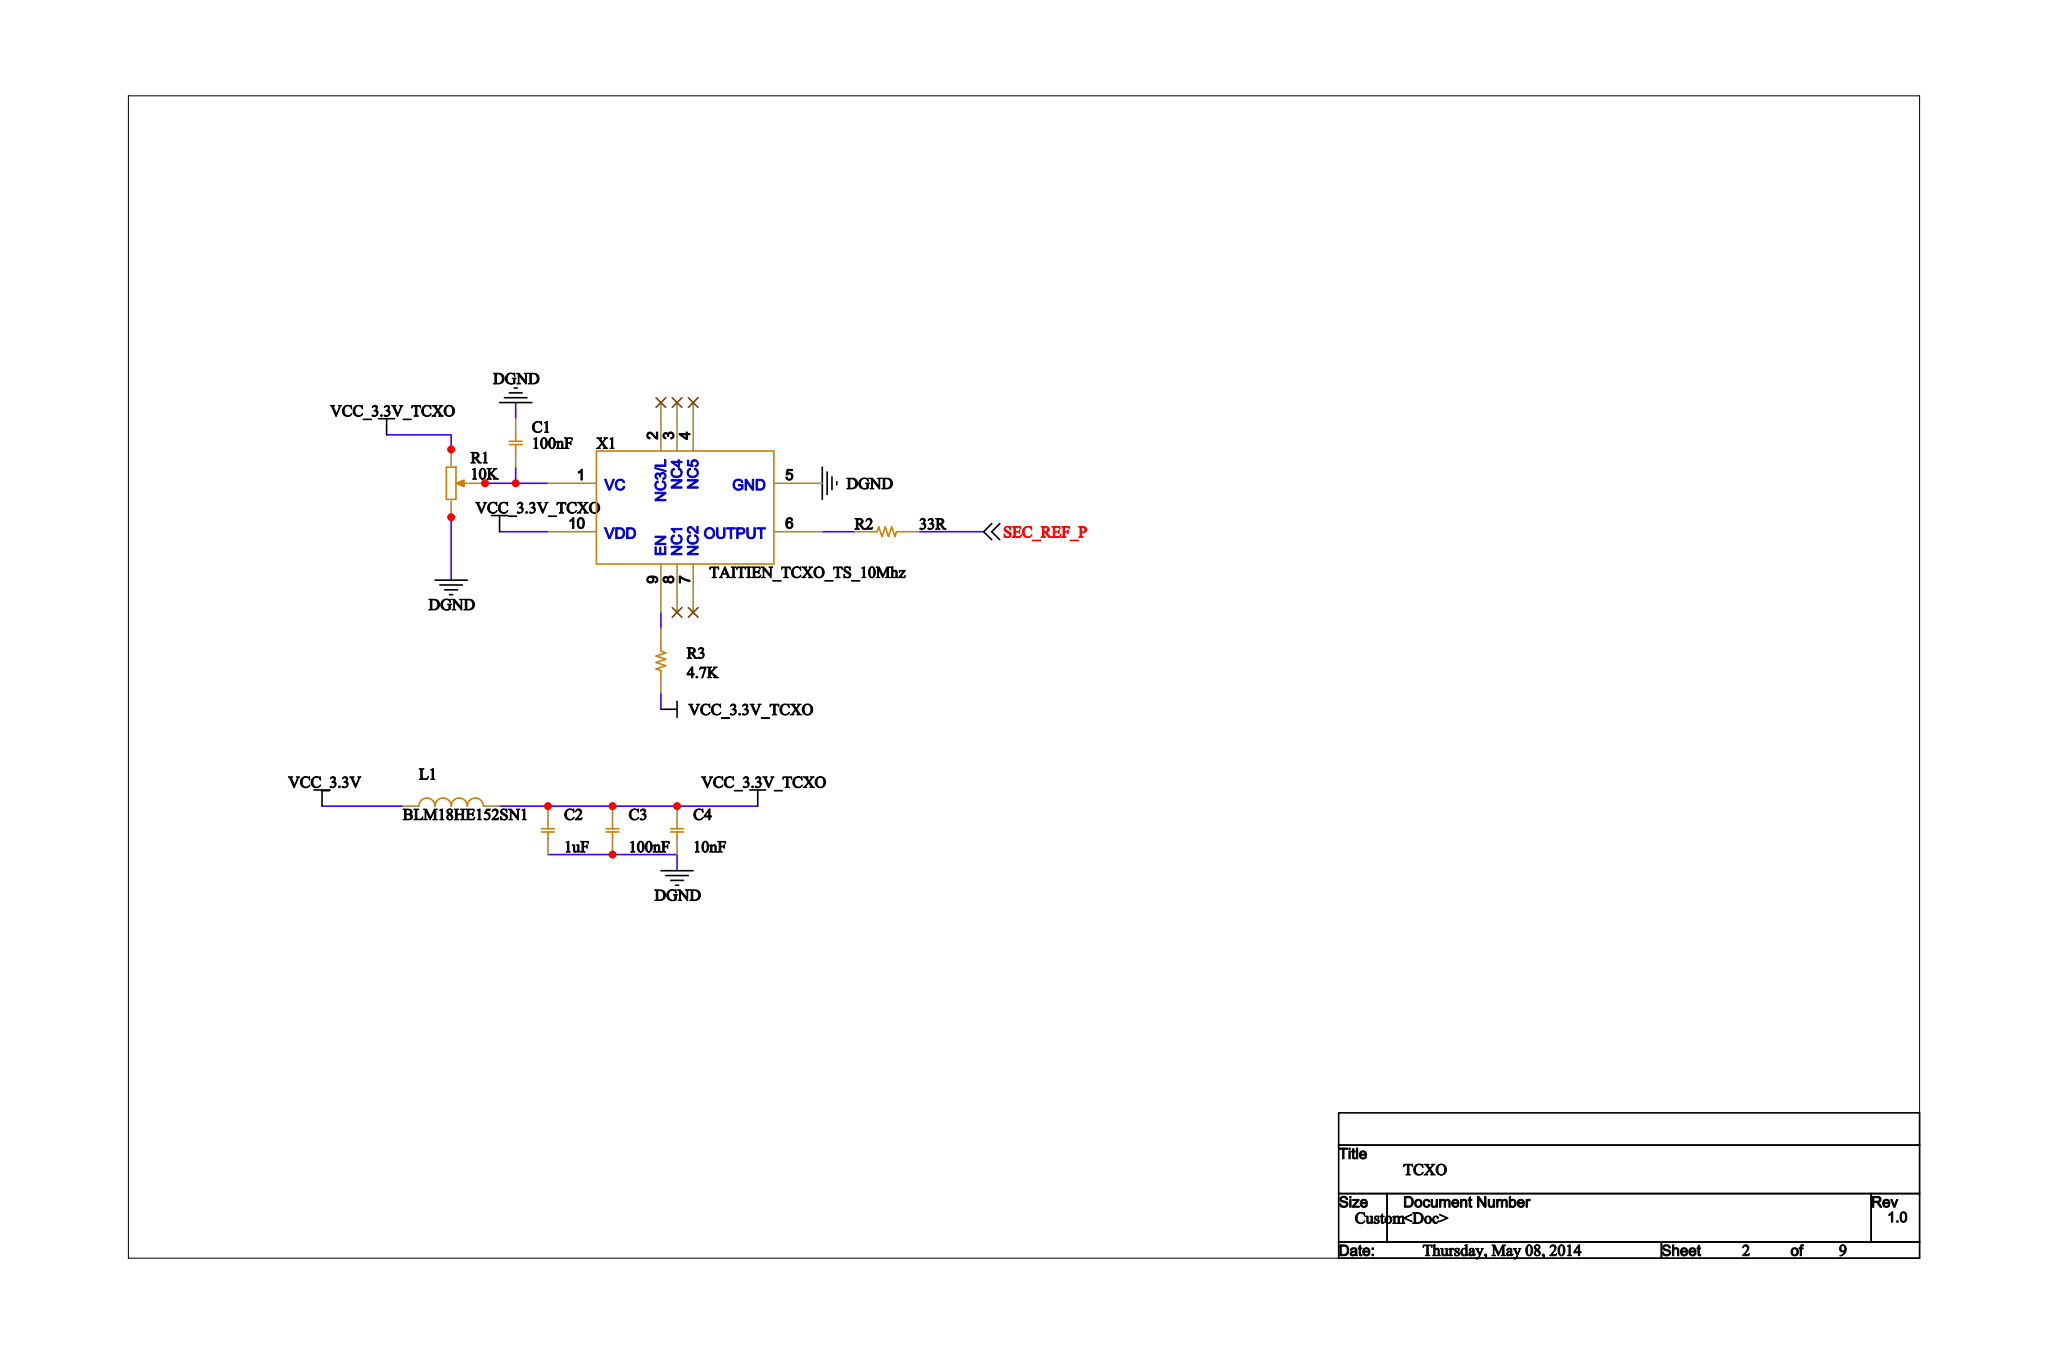Circuit board | Cadence Allegro | 233 parts | 224 nets | one sheet of the schematic
Parts on this sheet (reference | value | footprint):
C2 | 1uF | FPC-0402C
C3 | 100nF | FPC-0402C
C4 | 10nF | FPC-0402C
L1 | BLM18HE152SN1 | FPC-0603L
R1 | 10K | VR5
R2 | 33R | FPC-0603R
R3 | 4.7K | FPC-0603R
X1 | TAITIEN_TCXO_TS_10Mhz | FPC-CO10-5R0X7R0-S
Nets of these parts (net: part-pin ...):
DGND: C2-1 C3-1 C4-1 R1-2 X1-5
N68217: R1-3 X1-1
VCC_3.3V: L1-1
VCC_3.3V_TCXO: C2-2 C3-2 C4-2 L1-2 R1-1 R3-1 X1-10
N14985: R3-2 X1-9
N14969: R2-1 X1-6
SEC_REF_P: R2-2